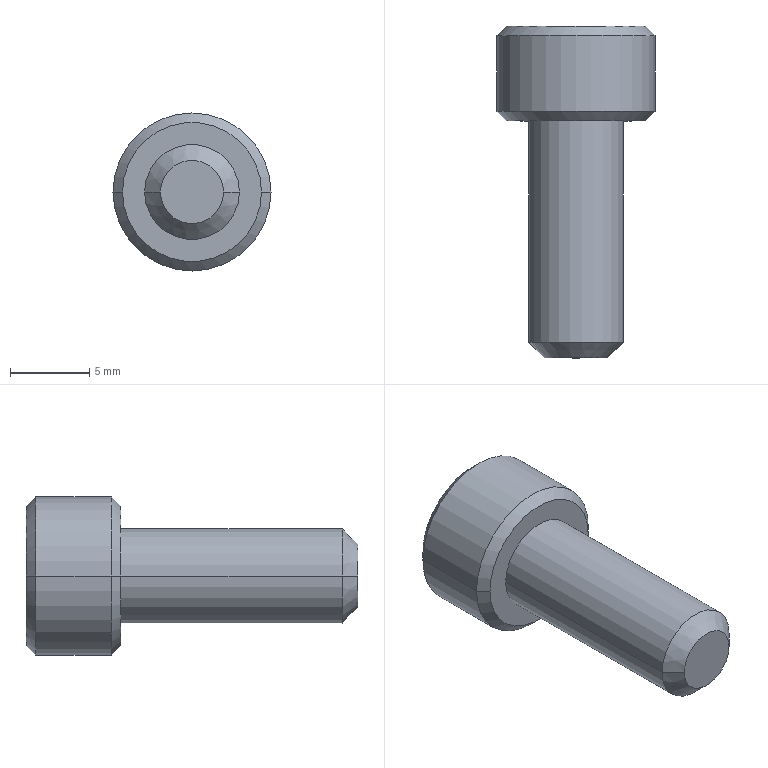Part | STEP file | BB62-M6-15L-7 | 1 solid | 27 faces | box 10 x 21 x 10 mm | volume 798.222 mm3 | plane 15 | cone 8 | cylinder 4 | commonest cylinder face diameters 6 x2 10 x2
STEP:
#1=CARTESIAN_POINT('',(0.,1.349,0.));
#2=VERTEX_POINT('',#1);
#3=CARTESIAN_POINT('',(2.86,3.,0.));
#4=VERTEX_POINT('',#3);
#5=CARTESIAN_POINT('',(0.,1.349,0.));
#6=DIRECTION('',(0.866,0.5,0.));
#7=VECTOR('',#6,1000.);
#8=LINE('',#5,#7);
#9=EDGE_CURVE('',#2,#4,#8,.T.);
#10=ORIENTED_EDGE('',*,*,#9,.F.);
#11=CARTESIAN_POINT('',(-2.86,3.,0.));
#12=VERTEX_POINT('',#11);
#13=CARTESIAN_POINT('',(0.,1.349,0.));
#14=DIRECTION('',(-0.866,0.5,0.));
#15=VECTOR('',#14,1000.);
#16=LINE('',#13,#15);
#17=EDGE_CURVE('',#2,#12,#16,.T.);
#18=ORIENTED_EDGE('',*,*,#17,.T.);
#19=CARTESIAN_POINT('',(-2.477,3.,1.43));
#20=VERTEX_POINT('',#19);
#21=CARTESIAN_POINT('',(0.,3.,0.));
#22=DIRECTION('',(0.,-1.,0.));
#23=DIRECTION('',(-1.,0.,0.));
#24=AXIS2_PLACEMENT_3D('',#21,#22,#23);
#25=CIRCLE('',#24,2.86);
#26=EDGE_CURVE('',#20,#12,#25,.T.);
#27=ORIENTED_EDGE('',*,*,#26,.F.);
#28=CARTESIAN_POINT('',(0.,3.,2.86));
#29=VERTEX_POINT('',#28);
#30=CARTESIAN_POINT('',(0.,3.,0.));
#31=DIRECTION('',(0.,-1.,0.));
#32=DIRECTION('',(-1.,0.,0.));
#33=AXIS2_PLACEMENT_3D('',#30,#31,#32);
#34=CIRCLE('',#33,2.86);
#35=EDGE_CURVE('',#29,#20,#34,.T.);
#36=ORIENTED_EDGE('',*,*,#35,.F.);
#37=CARTESIAN_POINT('',(2.477,3.,1.43));
#38=VERTEX_POINT('',#37);
#39=CARTESIAN_POINT('',(0.,3.,0.));
#40=DIRECTION('',(0.,-1.,0.));
#41=DIRECTION('',(-1.,0.,0.));
#42=AXIS2_PLACEMENT_3D('',#39,#40,#41);
#43=CIRCLE('',#42,2.86);
#44=EDGE_CURVE('',#38,#29,#43,.T.);
#45=ORIENTED_EDGE('',*,*,#44,.F.);
#46=CARTESIAN_POINT('',(0.,3.,0.));
#47=DIRECTION('',(0.,-1.,0.));
#48=DIRECTION('',(-1.,0.,0.));
#49=AXIS2_PLACEMENT_3D('',#46,#47,#48);
#50=CIRCLE('',#49,2.86);
#51=EDGE_CURVE('',#4,#38,#50,.T.);
#52=ORIENTED_EDGE('',*,*,#51,.F.);
#53=EDGE_LOOP('',(#10,#18,#27,#36,#45,#52));
#54=FACE_OUTER_BOUND('',#53,.T.);
#55=CARTESIAN_POINT('',(0.,1001.349,0.));
#56=DIRECTION('',(0.,1.,0.));
#57=DIRECTION('',(1.,0.,0.));
#58=AXIS2_PLACEMENT_3D('',#55,#56,#57);
#59=CONICAL_SURFACE('',#58,1732.051,1.047);
#60=ADVANCED_FACE('',(#54),#59,.F.);
#61=CARTESIAN_POINT('',(2.,-15.,0.));
#62=VERTEX_POINT('',#61);
#63=CARTESIAN_POINT('',(-2.,-15.,0.));
#64=VERTEX_POINT('',#63);
#65=CARTESIAN_POINT('',(0.,-15.,0.));
#66=DIRECTION('',(0.,1.,0.));
#67=DIRECTION('',(1.,0.,0.));
#68=AXIS2_PLACEMENT_3D('',#65,#66,#67);
#69=CIRCLE('',#68,2.);
#70=EDGE_CURVE('',#62,#64,#69,.T.);
#71=ORIENTED_EDGE('',*,*,#70,.T.);
#72=CARTESIAN_POINT('',(-3.,-14.,0.));
#73=VERTEX_POINT('',#72);
#74=CARTESIAN_POINT('',(-2.,-15.,0.));
#75=DIRECTION('',(-0.7071,0.7071,0.));
#76=VECTOR('',#75,1000.);
#77=LINE('',#74,#76);
#78=EDGE_CURVE('',#64,#73,#77,.T.);
#79=ORIENTED_EDGE('',*,*,#78,.T.);
#80=CARTESIAN_POINT('',(3.,-14.,0.));
#81=VERTEX_POINT('',#80);
#82=CARTESIAN_POINT('',(0.,-14.,0.));
#83=DIRECTION('',(0.,-1.,0.));
#84=DIRECTION('',(-1.,0.,0.));
#85=AXIS2_PLACEMENT_3D('',#82,#83,#84);
#86=CIRCLE('',#85,3.);
#87=EDGE_CURVE('',#73,#81,#86,.T.);
#88=ORIENTED_EDGE('',*,*,#87,.T.);
#89=CARTESIAN_POINT('',(2.,-15.,0.));
#90=DIRECTION('',(0.7071,0.7071,0.));
#91=VECTOR('',#90,1000.);
#92=LINE('',#89,#91);
#93=EDGE_CURVE('',#62,#81,#92,.T.);
#94=ORIENTED_EDGE('',*,*,#93,.F.);
#95=EDGE_LOOP('',(#71,#79,#88,#94));
#96=FACE_OUTER_BOUND('',#95,.T.);
#97=CARTESIAN_POINT('',(0.,-15.,0.));
#98=DIRECTION('',(0.,1.,0.));
#99=DIRECTION('',(1.,0.,0.));
#100=AXIS2_PLACEMENT_3D('',#97,#98,#99);
#101=CONICAL_SURFACE('',#100,2.,0.7854);
#102=ADVANCED_FACE('',(#96),#101,.T.);
#103=ORIENTED_EDGE('',*,*,#87,.F.);
#104=CARTESIAN_POINT('',(-3.,0.,0.));
#105=VERTEX_POINT('',#104);
#106=CARTESIAN_POINT('',(-3.,-14.,0.));
#107=DIRECTION('',(0.,1.,0.));
#108=VECTOR('',#107,1000.);
#109=LINE('',#106,#108);
#110=EDGE_CURVE('',#73,#105,#109,.T.);
#111=ORIENTED_EDGE('',*,*,#110,.T.);
#112=CARTESIAN_POINT('',(3.,0.,0.));
#113=VERTEX_POINT('',#112);
#114=CARTESIAN_POINT('',(0.,0.,0.));
#115=DIRECTION('',(0.,-1.,0.));
#116=DIRECTION('',(-1.,0.,0.));
#117=AXIS2_PLACEMENT_3D('',#114,#115,#116);
#118=CIRCLE('',#117,3.);
#119=EDGE_CURVE('',#105,#113,#118,.T.);
#120=ORIENTED_EDGE('',*,*,#119,.T.);
#121=CARTESIAN_POINT('',(3.,-14.,0.));
#122=DIRECTION('',(0.,1.,0.));
#123=VECTOR('',#122,1000.);
#124=LINE('',#121,#123);
#125=EDGE_CURVE('',#81,#113,#124,.T.);
#126=ORIENTED_EDGE('',*,*,#125,.F.);
#127=EDGE_LOOP('',(#103,#111,#120,#126));
#128=FACE_OUTER_BOUND('',#127,.T.);
#129=CARTESIAN_POINT('',(0.,-14.,0.));
#130=DIRECTION('',(0.,1.,0.));
#131=DIRECTION('',(1.,0.,0.));
#132=AXIS2_PLACEMENT_3D('',#129,#130,#131);
#133=CYLINDRICAL_SURFACE('',#132,3.);
#134=ADVANCED_FACE('',(#128),#133,.T.);
#135=CARTESIAN_POINT('',(-4.4,6.,0.));
#136=VERTEX_POINT('',#135);
#137=CARTESIAN_POINT('',(4.4,6.,0.));
#138=VERTEX_POINT('',#137);
#139=CARTESIAN_POINT('',(0.,6.,0.));
#140=DIRECTION('',(0.,-1.,0.));
#141=DIRECTION('',(-1.,0.,0.));
#142=AXIS2_PLACEMENT_3D('',#139,#140,#141);
#143=CIRCLE('',#142,4.4);
#144=EDGE_CURVE('',#136,#138,#143,.T.);
#145=ORIENTED_EDGE('',*,*,#144,.T.);
#146=CARTESIAN_POINT('',(5.,5.4,0.));
#147=VERTEX_POINT('',#146);
#148=CARTESIAN_POINT('',(5.,5.4,0.));
#149=DIRECTION('',(0.7071,-0.7071,0.));
#150=VECTOR('',#149,1000.);
#151=LINE('',#148,#150);
#152=EDGE_CURVE('',#138,#147,#151,.T.);
#153=ORIENTED_EDGE('',*,*,#152,.T.);
#154=CARTESIAN_POINT('',(-5.,5.4,0.));
#155=VERTEX_POINT('',#154);
#156=CARTESIAN_POINT('',(0.,5.4,0.));
#157=DIRECTION('',(0.,-1.,0.));
#158=DIRECTION('',(-1.,0.,0.));
#159=AXIS2_PLACEMENT_3D('',#156,#157,#158);
#160=CIRCLE('',#159,5.);
#161=EDGE_CURVE('',#155,#147,#160,.T.);
#162=ORIENTED_EDGE('',*,*,#161,.F.);
#163=CARTESIAN_POINT('',(-5.,5.4,0.));
#164=DIRECTION('',(-0.7071,-0.7071,0.));
#165=VECTOR('',#164,1000.);
#166=LINE('',#163,#165);
#167=EDGE_CURVE('',#136,#155,#166,.T.);
#168=ORIENTED_EDGE('',*,*,#167,.F.);
#169=EDGE_LOOP('',(#145,#153,#162,#168));
#170=FACE_OUTER_BOUND('',#169,.T.);
#171=CARTESIAN_POINT('',(0.,5.4,0.));
#172=DIRECTION('',(0.,-1.,0.));
#173=DIRECTION('',(-1.,0.,0.));
#174=AXIS2_PLACEMENT_3D('',#171,#172,#173);
#175=CONICAL_SURFACE('',#174,5.,0.7854);
#176=ADVANCED_FACE('',(#170),#175,.T.);
#177=ORIENTED_EDGE('',*,*,#161,.T.);
#178=CARTESIAN_POINT('',(5.,0.6,0.));
#179=VERTEX_POINT('',#178);
#180=CARTESIAN_POINT('',(5.,1.62,0.));
#181=DIRECTION('',(0.,-1.,0.));
#182=VECTOR('',#181,1000.);
#183=LINE('',#180,#182);
#184=EDGE_CURVE('',#147,#179,#183,.T.);
#185=ORIENTED_EDGE('',*,*,#184,.T.);
#186=CARTESIAN_POINT('',(-5.,0.6,0.));
#187=VERTEX_POINT('',#186);
#188=CARTESIAN_POINT('',(0.,0.6,0.));
#189=DIRECTION('',(0.,-1.,0.));
#190=DIRECTION('',(-1.,0.,0.));
#191=AXIS2_PLACEMENT_3D('',#188,#189,#190);
#192=CIRCLE('',#191,5.);
#193=EDGE_CURVE('',#187,#179,#192,.T.);
#194=ORIENTED_EDGE('',*,*,#193,.F.);
#195=CARTESIAN_POINT('',(-5.,1.62,0.));
#196=DIRECTION('',(0.,-1.,0.));
#197=VECTOR('',#196,1000.);
#198=LINE('',#195,#197);
#199=EDGE_CURVE('',#155,#187,#198,.T.);
#200=ORIENTED_EDGE('',*,*,#199,.F.);
#201=EDGE_LOOP('',(#177,#185,#194,#200));
#202=FACE_OUTER_BOUND('',#201,.T.);
#203=CARTESIAN_POINT('',(0.,1.62,0.));
#204=DIRECTION('',(0.,-1.,0.));
#205=DIRECTION('',(-1.,0.,0.));
#206=AXIS2_PLACEMENT_3D('',#203,#204,#205);
#207=CYLINDRICAL_SURFACE('',#206,5.);
#208=ADVANCED_FACE('',(#202),#207,.T.);
#209=CARTESIAN_POINT('',(-4.4,0.,0.));
#210=VERTEX_POINT('',#209);
#211=CARTESIAN_POINT('',(4.4,0.,0.));
#212=VERTEX_POINT('',#211);
#213=CARTESIAN_POINT('',(0.,0.,0.));
#214=DIRECTION('',(0.,-1.,0.));
#215=DIRECTION('',(-1.,0.,0.));
#216=AXIS2_PLACEMENT_3D('',#213,#214,#215);
#217=CIRCLE('',#216,4.4);
#218=EDGE_CURVE('',#210,#212,#217,.T.);
#219=ORIENTED_EDGE('',*,*,#218,.F.);
#220=CARTESIAN_POINT('',(-4.4,0.,0.));
#221=DIRECTION('',(-0.7071,0.7071,0.));
#222=VECTOR('',#221,1000.);
#223=LINE('',#220,#222);
#224=EDGE_CURVE('',#210,#187,#223,.T.);
#225=ORIENTED_EDGE('',*,*,#224,.T.);
#226=ORIENTED_EDGE('',*,*,#193,.T.);
#227=CARTESIAN_POINT('',(4.4,0.,0.));
#228=DIRECTION('',(0.7071,0.7071,0.));
#229=VECTOR('',#228,1000.);
#230=LINE('',#227,#229);
#231=EDGE_CURVE('',#212,#179,#230,.T.);
#232=ORIENTED_EDGE('',*,*,#231,.F.);
#233=EDGE_LOOP('',(#219,#225,#226,#232));
#234=FACE_OUTER_BOUND('',#233,.T.);
#235=CARTESIAN_POINT('',(0.,0.,0.));
#236=DIRECTION('',(0.,1.,0.));
#237=DIRECTION('',(1.,0.,0.));
#238=AXIS2_PLACEMENT_3D('',#235,#236,#237);
#239=CONICAL_SURFACE('',#238,4.4,0.7854);
#240=ADVANCED_FACE('',(#234),#239,.T.);
#241=ORIENTED_EDGE('',*,*,#144,.F.);
#242=CARTESIAN_POINT('',(0.,6.,0.));
#243=DIRECTION('',(0.,-1.,0.));
#244=DIRECTION('',(-1.,0.,0.));
#245=AXIS2_PLACEMENT_3D('',#242,#243,#244);
#246=CIRCLE('',#245,4.4);
#247=EDGE_CURVE('',#138,#136,#246,.T.);
#248=ORIENTED_EDGE('',*,*,#247,.F.);
#249=EDGE_LOOP('',(#241,#248));
#250=FACE_OUTER_BOUND('',#249,.T.);
#251=CARTESIAN_POINT('',(0.,6.,-2.86));
#252=VERTEX_POINT('',#251);
#253=CARTESIAN_POINT('',(-2.477,6.,-1.43));
#254=VERTEX_POINT('',#253);
#255=CARTESIAN_POINT('',(0.,6.,-2.86));
#256=DIRECTION('',(-0.866,0.,0.5));
#257=VECTOR('',#256,1000.);
#258=LINE('',#255,#257);
#259=EDGE_CURVE('',#252,#254,#258,.T.);
#260=ORIENTED_EDGE('',*,*,#259,.F.);
#261=CARTESIAN_POINT('',(2.477,6.,-1.43));
#262=VERTEX_POINT('',#261);
#263=CARTESIAN_POINT('',(2.477,6.,-1.43));
#264=DIRECTION('',(-0.866,0.,-0.5));
#265=VECTOR('',#264,1000.);
#266=LINE('',#263,#265);
#267=EDGE_CURVE('',#262,#252,#266,.T.);
#268=ORIENTED_EDGE('',*,*,#267,.F.);
#269=CARTESIAN_POINT('',(2.477,6.,1.43));
#270=VERTEX_POINT('',#269);
#271=CARTESIAN_POINT('',(2.477,6.,1.43));
#272=DIRECTION('',(0.,0.,-1.));
#273=VECTOR('',#272,1000.);
#274=LINE('',#271,#273);
#275=EDGE_CURVE('',#270,#262,#274,.T.);
#276=ORIENTED_EDGE('',*,*,#275,.F.);
#277=CARTESIAN_POINT('',(0.,6.,2.86));
#278=VERTEX_POINT('',#277);
#279=CARTESIAN_POINT('',(0.,6.,2.86));
#280=DIRECTION('',(0.866,0.,-0.5));
#281=VECTOR('',#280,1000.);
#282=LINE('',#279,#281);
#283=EDGE_CURVE('',#278,#270,#282,.T.);
#284=ORIENTED_EDGE('',*,*,#283,.F.);
#285=CARTESIAN_POINT('',(-2.477,6.,1.43));
#286=VERTEX_POINT('',#285);
#287=CARTESIAN_POINT('',(-2.477,6.,1.43));
#288=DIRECTION('',(0.866,0.,0.5));
#289=VECTOR('',#288,1000.);
#290=LINE('',#287,#289);
#291=EDGE_CURVE('',#286,#278,#290,.T.);
#292=ORIENTED_EDGE('',*,*,#291,.F.);
#293=CARTESIAN_POINT('',(-2.477,6.,-1.43));
#294=DIRECTION('',(0.,0.,1.));
#295=VECTOR('',#294,1000.);
#296=LINE('',#293,#295);
#297=EDGE_CURVE('',#254,#286,#296,.T.);
#298=ORIENTED_EDGE('',*,*,#297,.F.);
#299=EDGE_LOOP('',(#260,#268,#276,#284,#292,#298));
#300=FACE_BOUND('',#299,.T.);
#301=CARTESIAN_POINT('',(4.4,6.,0.));
#302=DIRECTION('',(0.,1.,0.));
#303=DIRECTION('',(1.,0.,0.));
#304=AXIS2_PLACEMENT_3D('',#301,#302,#303);
#305=PLANE('',#304);
#306=ADVANCED_FACE('',(#250,#300),#305,.T.);
#307=CARTESIAN_POINT('',(0.,0.,0.));
#308=DIRECTION('',(0.,-1.,0.));
#309=DIRECTION('',(-1.,0.,0.));
#310=AXIS2_PLACEMENT_3D('',#307,#308,#309);
#311=CIRCLE('',#310,3.);
#312=EDGE_CURVE('',#113,#105,#311,.T.);
#313=ORIENTED_EDGE('',*,*,#312,.F.);
#314=ORIENTED_EDGE('',*,*,#119,.F.);
#315=EDGE_LOOP('',(#313,#314));
#316=FACE_BOUND('',#315,.T.);
#317=CARTESIAN_POINT('',(0.,0.,0.));
#318=DIRECTION('',(0.,-1.,0.));
#319=DIRECTION('',(-1.,0.,0.));
#320=AXIS2_PLACEMENT_3D('',#317,#318,#319);
#321=CIRCLE('',#320,4.4);
#322=EDGE_CURVE('',#212,#210,#321,.T.);
#323=ORIENTED_EDGE('',*,*,#322,.T.);
#324=ORIENTED_EDGE('',*,*,#218,.T.);
#325=EDGE_LOOP('',(#323,#324));
#326=FACE_OUTER_BOUND('',#325,.T.);
#327=CARTESIAN_POINT('',(0.,0.,0.));
#328=DIRECTION('',(0.,-1.,0.));
#329=DIRECTION('',(-1.,0.,0.));
#330=AXIS2_PLACEMENT_3D('',#327,#328,#329);
#331=PLANE('',#330);
#332=ADVANCED_FACE('',(#316,#326),#331,.T.);
#333=ORIENTED_EDGE('',*,*,#224,.F.);
#334=ORIENTED_EDGE('',*,*,#322,.F.);
#335=ORIENTED_EDGE('',*,*,#231,.T.);
#336=CARTESIAN_POINT('',(0.,0.6,0.));
#337=DIRECTION('',(0.,-1.,0.));
#338=DIRECTION('',(-1.,0.,0.));
#339=AXIS2_PLACEMENT_3D('',#336,#337,#338);
#340=CIRCLE('',#339,5.);
#341=EDGE_CURVE('',#179,#187,#340,.T.);
#342=ORIENTED_EDGE('',*,*,#341,.T.);
#343=EDGE_LOOP('',(#333,#334,#335,#342));
#344=FACE_OUTER_BOUND('',#343,.T.);
#345=CARTESIAN_POINT('',(0.,0.,0.));
#346=DIRECTION('',(0.,1.,0.));
#347=DIRECTION('',(1.,0.,0.));
#348=AXIS2_PLACEMENT_3D('',#345,#346,#347);
#349=CONICAL_SURFACE('',#348,4.4,0.7854);
#350=ADVANCED_FACE('',(#344),#349,.T.);
#351=ORIENTED_EDGE('',*,*,#184,.F.);
#352=CARTESIAN_POINT('',(0.,5.4,0.));
#353=DIRECTION('',(0.,-1.,0.));
#354=DIRECTION('',(-1.,0.,0.));
#355=AXIS2_PLACEMENT_3D('',#352,#353,#354);
#356=CIRCLE('',#355,5.);
#357=EDGE_CURVE('',#147,#155,#356,.T.);
#358=ORIENTED_EDGE('',*,*,#357,.T.);
#359=ORIENTED_EDGE('',*,*,#199,.T.);
#360=ORIENTED_EDGE('',*,*,#341,.F.);
#361=EDGE_LOOP('',(#351,#358,#359,#360));
#362=FACE_OUTER_BOUND('',#361,.T.);
#363=CARTESIAN_POINT('',(0.,1.62,0.));
#364=DIRECTION('',(0.,-1.,0.));
#365=DIRECTION('',(-1.,0.,0.));
#366=AXIS2_PLACEMENT_3D('',#363,#364,#365);
#367=CYLINDRICAL_SURFACE('',#366,5.);
#368=ADVANCED_FACE('',(#362),#367,.T.);
#369=ORIENTED_EDGE('',*,*,#152,.F.);
#370=ORIENTED_EDGE('',*,*,#247,.T.);
#371=ORIENTED_EDGE('',*,*,#167,.T.);
#372=ORIENTED_EDGE('',*,*,#357,.F.);
#373=EDGE_LOOP('',(#369,#370,#371,#372));
#374=FACE_OUTER_BOUND('',#373,.T.);
#375=CARTESIAN_POINT('',(0.,5.4,0.));
#376=DIRECTION('',(0.,-1.,0.));
#377=DIRECTION('',(-1.,0.,0.));
#378=AXIS2_PLACEMENT_3D('',#375,#376,#377);
#379=CONICAL_SURFACE('',#378,5.,0.7854);
#380=ADVANCED_FACE('',(#374),#379,.T.);
#381=ORIENTED_EDGE('',*,*,#110,.F.);
#382=CARTESIAN_POINT('',(0.,-14.,0.));
#383=DIRECTION('',(0.,-1.,0.));
#384=DIRECTION('',(-1.,0.,0.));
#385=AXIS2_PLACEMENT_3D('',#382,#383,#384);
#386=CIRCLE('',#385,3.);
#387=EDGE_CURVE('',#81,#73,#386,.T.);
#388=ORIENTED_EDGE('',*,*,#387,.F.);
#389=ORIENTED_EDGE('',*,*,#125,.T.);
#390=ORIENTED_EDGE('',*,*,#312,.T.);
#391=EDGE_LOOP('',(#381,#388,#389,#390));
#392=FACE_OUTER_BOUND('',#391,.T.);
#393=CARTESIAN_POINT('',(0.,-14.,0.));
#394=DIRECTION('',(0.,1.,0.));
#395=DIRECTION('',(1.,0.,0.));
#396=AXIS2_PLACEMENT_3D('',#393,#394,#395);
#397=CYLINDRICAL_SURFACE('',#396,3.);
#398=ADVANCED_FACE('',(#392),#397,.T.);
#399=ORIENTED_EDGE('',*,*,#70,.F.);
#400=CARTESIAN_POINT('',(0.,-15.,0.));
#401=DIRECTION('',(0.,1.,0.));
#402=DIRECTION('',(1.,0.,0.));
#403=AXIS2_PLACEMENT_3D('',#400,#401,#402);
#404=CIRCLE('',#403,2.);
#405=EDGE_CURVE('',#64,#62,#404,.T.);
#406=ORIENTED_EDGE('',*,*,#405,.F.);
#407=EDGE_LOOP('',(#399,#406));
#408=FACE_OUTER_BOUND('',#407,.T.);
#409=CARTESIAN_POINT('',(0.,-15.,0.));
#410=DIRECTION('',(0.,-1.,0.));
#411=DIRECTION('',(-1.,0.,0.));
#412=AXIS2_PLACEMENT_3D('',#409,#410,#411);
#413=PLANE('',#412);
#414=ADVANCED_FACE('',(#408),#413,.T.);
#415=ORIENTED_EDGE('',*,*,#78,.F.);
#416=ORIENTED_EDGE('',*,*,#405,.T.);
#417=ORIENTED_EDGE('',*,*,#93,.T.);
#418=ORIENTED_EDGE('',*,*,#387,.T.);
#419=EDGE_LOOP('',(#415,#416,#417,#418));
#420=FACE_OUTER_BOUND('',#419,.T.);
#421=CARTESIAN_POINT('',(0.,-15.,0.));
#422=DIRECTION('',(0.,1.,0.));
#423=DIRECTION('',(1.,0.,0.));
#424=AXIS2_PLACEMENT_3D('',#421,#422,#423);
#425=CONICAL_SURFACE('',#424,2.,0.7854);
#426=ADVANCED_FACE('',(#420),#425,.T.);
#427=CARTESIAN_POINT('',(2.477,3.,-1.43));
#428=VERTEX_POINT('',#427);
#429=CARTESIAN_POINT('',(0.,3.,-2.86));
#430=VERTEX_POINT('',#429);
#431=CARTESIAN_POINT('',(2.477,3.,-1.43));
#432=DIRECTION('',(-0.866,0.,-0.5));
#433=VECTOR('',#432,1000.);
#434=LINE('',#431,#433);
#435=EDGE_CURVE('',#428,#430,#434,.T.);
#436=ORIENTED_EDGE('',*,*,#435,.F.);
#437=CARTESIAN_POINT('',(2.477,6.,-1.43));
#438=DIRECTION('',(0.,-1.,0.));
#439=VECTOR('',#438,1000.);
#440=LINE('',#437,#439);
#441=EDGE_CURVE('',#262,#428,#440,.T.);
#442=ORIENTED_EDGE('',*,*,#441,.F.);
#443=ORIENTED_EDGE('',*,*,#267,.T.);
#444=CARTESIAN_POINT('',(0.,6.,-2.86));
#445=DIRECTION('',(0.,-1.,0.));
#446=VECTOR('',#445,1000.);
#447=LINE('',#444,#446);
#448=EDGE_CURVE('',#252,#430,#447,.T.);
#449=ORIENTED_EDGE('',*,*,#448,.T.);
#450=EDGE_LOOP('',(#436,#442,#443,#449));
#451=FACE_OUTER_BOUND('',#450,.T.);
#452=CARTESIAN_POINT('',(2.477,6.,-1.43));
#453=DIRECTION('',(-0.5,0.,0.866));
#454=DIRECTION('',(0.866,0.,0.5));
#455=AXIS2_PLACEMENT_3D('',#452,#453,#454);
#456=PLANE('',#455);
#457=ADVANCED_FACE('',(#451),#456,.T.);
#458=CARTESIAN_POINT('',(-2.477,3.,-1.43));
#459=VERTEX_POINT('',#458);
#460=CARTESIAN_POINT('',(0.,3.,-2.86));
#461=DIRECTION('',(-0.866,0.,0.5));
#462=VECTOR('',#461,1000.);
#463=LINE('',#460,#462);
#464=EDGE_CURVE('',#430,#459,#463,.T.);
#465=ORIENTED_EDGE('',*,*,#464,.F.);
#466=ORIENTED_EDGE('',*,*,#448,.F.);
#467=ORIENTED_EDGE('',*,*,#259,.T.);
#468=CARTESIAN_POINT('',(-2.477,6.,-1.43));
#469=DIRECTION('',(0.,-1.,0.));
#470=VECTOR('',#469,1000.);
#471=LINE('',#468,#470);
#472=EDGE_CURVE('',#254,#459,#471,.T.);
#473=ORIENTED_EDGE('',*,*,#472,.T.);
#474=EDGE_LOOP('',(#465,#466,#467,#473));
#475=FACE_OUTER_BOUND('',#474,.T.);
#476=CARTESIAN_POINT('',(0.,6.,-2.86));
#477=DIRECTION('',(0.5,0.,0.866));
#478=DIRECTION('',(0.866,0.,-0.5));
#479=AXIS2_PLACEMENT_3D('',#476,#477,#478);
#480=PLANE('',#479);
#481=ADVANCED_FACE('',(#475),#480,.T.);
#482=CARTESIAN_POINT('',(-2.477,3.,-1.43));
#483=DIRECTION('',(0.,0.,1.));
#484=VECTOR('',#483,1000.);
#485=LINE('',#482,#484);
#486=EDGE_CURVE('',#459,#20,#485,.T.);
#487=ORIENTED_EDGE('',*,*,#486,.F.);
#488=ORIENTED_EDGE('',*,*,#472,.F.);
#489=ORIENTED_EDGE('',*,*,#297,.T.);
#490=CARTESIAN_POINT('',(-2.477,6.,1.43));
#491=DIRECTION('',(0.,-1.,0.));
#492=VECTOR('',#491,1000.);
#493=LINE('',#490,#492);
#494=EDGE_CURVE('',#286,#20,#493,.T.);
#495=ORIENTED_EDGE('',*,*,#494,.T.);
#496=EDGE_LOOP('',(#487,#488,#489,#495));
#497=FACE_OUTER_BOUND('',#496,.T.);
#498=CARTESIAN_POINT('',(-2.477,6.,-1.43));
#499=DIRECTION('',(1.,0.,0.));
#500=DIRECTION('',(0.,0.,-1.));
#501=AXIS2_PLACEMENT_3D('',#498,#499,#500);
#502=PLANE('',#501);
#503=ADVANCED_FACE('',(#497),#502,.T.);
#504=CARTESIAN_POINT('',(-2.477,3.,1.43));
#505=DIRECTION('',(0.866,0.,0.5));
#506=VECTOR('',#505,1000.);
#507=LINE('',#504,#506);
#508=EDGE_CURVE('',#20,#29,#507,.T.);
#509=ORIENTED_EDGE('',*,*,#508,.F.);
#510=ORIENTED_EDGE('',*,*,#494,.F.);
#511=ORIENTED_EDGE('',*,*,#291,.T.);
#512=CARTESIAN_POINT('',(0.,6.,2.86));
#513=DIRECTION('',(0.,-1.,0.));
#514=VECTOR('',#513,1000.);
#515=LINE('',#512,#514);
#516=EDGE_CURVE('',#278,#29,#515,.T.);
#517=ORIENTED_EDGE('',*,*,#516,.T.);
#518=EDGE_LOOP('',(#509,#510,#511,#517));
#519=FACE_OUTER_BOUND('',#518,.T.);
#520=CARTESIAN_POINT('',(-2.477,6.,1.43));
#521=DIRECTION('',(0.5,0.,-0.866));
#522=DIRECTION('',(-0.866,0.,-0.5));
#523=AXIS2_PLACEMENT_3D('',#520,#521,#522);
#524=PLANE('',#523);
#525=ADVANCED_FACE('',(#519),#524,.T.);
#526=CARTESIAN_POINT('',(0.,3.,2.86));
#527=DIRECTION('',(0.866,0.,-0.5));
#528=VECTOR('',#527,1000.);
#529=LINE('',#526,#528);
#530=EDGE_CURVE('',#29,#38,#529,.T.);
#531=ORIENTED_EDGE('',*,*,#530,.F.);
#532=ORIENTED_EDGE('',*,*,#516,.F.);
#533=ORIENTED_EDGE('',*,*,#283,.T.);
#534=CARTESIAN_POINT('',(2.477,6.,1.43));
#535=DIRECTION('',(0.,-1.,0.));
#536=VECTOR('',#535,1000.);
#537=LINE('',#534,#536);
#538=EDGE_CURVE('',#270,#38,#537,.T.);
#539=ORIENTED_EDGE('',*,*,#538,.T.);
#540=EDGE_LOOP('',(#531,#532,#533,#539));
#541=FACE_OUTER_BOUND('',#540,.T.);
#542=CARTESIAN_POINT('',(0.,6.,2.86));
#543=DIRECTION('',(-0.5,0.,-0.866));
#544=DIRECTION('',(-0.866,0.,0.5));
#545=AXIS2_PLACEMENT_3D('',#542,#543,#544);
#546=PLANE('',#545);
#547=ADVANCED_FACE('',(#541),#546,.T.);
#548=CARTESIAN_POINT('',(2.477,3.,1.43));
#549=DIRECTION('',(0.,0.,-1.));
#550=VECTOR('',#549,1000.);
#551=LINE('',#548,#550);
#552=EDGE_CURVE('',#38,#428,#551,.T.);
#553=ORIENTED_EDGE('',*,*,#552,.F.);
#554=ORIENTED_EDGE('',*,*,#538,.F.);
#555=ORIENTED_EDGE('',*,*,#275,.T.);
#556=ORIENTED_EDGE('',*,*,#441,.T.);
#557=EDGE_LOOP('',(#553,#554,#555,#556));
#558=FACE_OUTER_BOUND('',#557,.T.);
#559=CARTESIAN_POINT('',(2.477,6.,1.43));
#560=DIRECTION('',(-1.,0.,0.));
#561=DIRECTION('',(0.,0.,1.));
#562=AXIS2_PLACEMENT_3D('',#559,#560,#561);
#563=PLANE('',#562);
#564=ADVANCED_FACE('',(#558),#563,.T.);
#565=ORIENTED_EDGE('',*,*,#435,.T.);
#566=CARTESIAN_POINT('',(0.,3.,0.));
#567=DIRECTION('',(0.,-1.,0.));
#568=DIRECTION('',(-1.,0.,0.));
#569=AXIS2_PLACEMENT_3D('',#566,#567,#568);
#570=CIRCLE('',#569,2.86);
#571=EDGE_CURVE('',#430,#428,#570,.T.);
#572=ORIENTED_EDGE('',*,*,#571,.T.);
#573=EDGE_LOOP('',(#565,#572));
#574=FACE_OUTER_BOUND('',#573,.T.);
#575=CARTESIAN_POINT('',(0.,3.,0.));
#576=DIRECTION('',(0.,1.,0.));
#577=DIRECTION('',(1.,0.,0.));
#578=AXIS2_PLACEMENT_3D('',#575,#576,#577);
#579=PLANE('',#578);
#580=ADVANCED_FACE('',(#574),#579,.F.);
#581=ORIENTED_EDGE('',*,*,#552,.T.);
#582=CARTESIAN_POINT('',(0.,3.,0.));
#583=DIRECTION('',(0.,-1.,0.));
#584=DIRECTION('',(-1.,0.,0.));
#585=AXIS2_PLACEMENT_3D('',#582,#583,#584);
#586=CIRCLE('',#585,2.86);
#587=EDGE_CURVE('',#428,#4,#586,.T.);
#588=ORIENTED_EDGE('',*,*,#587,.T.);
#589=ORIENTED_EDGE('',*,*,#51,.T.);
#590=EDGE_LOOP('',(#581,#588,#589));
#591=FACE_OUTER_BOUND('',#590,.T.);
#592=CARTESIAN_POINT('',(0.,3.,0.));
#593=DIRECTION('',(0.,1.,0.));
#594=DIRECTION('',(1.,0.,0.));
#595=AXIS2_PLACEMENT_3D('',#592,#593,#594);
#596=PLANE('',#595);
#597=ADVANCED_FACE('',(#591),#596,.F.);
#598=ORIENTED_EDGE('',*,*,#530,.T.);
#599=ORIENTED_EDGE('',*,*,#44,.T.);
#600=EDGE_LOOP('',(#598,#599));
#601=FACE_OUTER_BOUND('',#600,.T.);
#602=CARTESIAN_POINT('',(0.,3.,0.));
#603=DIRECTION('',(0.,1.,0.));
#604=DIRECTION('',(1.,0.,0.));
#605=AXIS2_PLACEMENT_3D('',#602,#603,#604);
#606=PLANE('',#605);
#607=ADVANCED_FACE('',(#601),#606,.F.);
#608=ORIENTED_EDGE('',*,*,#508,.T.);
#609=ORIENTED_EDGE('',*,*,#35,.T.);
#610=EDGE_LOOP('',(#608,#609));
#611=FACE_OUTER_BOUND('',#610,.T.);
#612=CARTESIAN_POINT('',(0.,3.,0.));
#613=DIRECTION('',(0.,1.,0.));
#614=DIRECTION('',(1.,0.,0.));
#615=AXIS2_PLACEMENT_3D('',#612,#613,#614);
#616=PLANE('',#615);
#617=ADVANCED_FACE('',(#611),#616,.F.);
#618=ORIENTED_EDGE('',*,*,#486,.T.);
#619=ORIENTED_EDGE('',*,*,#26,.T.);
#620=CARTESIAN_POINT('',(0.,3.,0.));
#621=DIRECTION('',(0.,-1.,0.));
#622=DIRECTION('',(-1.,0.,0.));
#623=AXIS2_PLACEMENT_3D('',#620,#621,#622);
#624=CIRCLE('',#623,2.86);
#625=EDGE_CURVE('',#12,#459,#624,.T.);
#626=ORIENTED_EDGE('',*,*,#625,.T.);
#627=EDGE_LOOP('',(#618,#619,#626));
#628=FACE_OUTER_BOUND('',#627,.T.);
#629=CARTESIAN_POINT('',(0.,3.,0.));
#630=DIRECTION('',(0.,1.,0.));
#631=DIRECTION('',(1.,0.,0.));
#632=AXIS2_PLACEMENT_3D('',#629,#630,#631);
#633=PLANE('',#632);
#634=ADVANCED_FACE('',(#628),#633,.F.);
#635=ORIENTED_EDGE('',*,*,#464,.T.);
#636=CARTESIAN_POINT('',(0.,3.,0.));
#637=DIRECTION('',(0.,-1.,0.));
#638=DIRECTION('',(-1.,0.,0.));
#639=AXIS2_PLACEMENT_3D('',#636,#637,#638);
#640=CIRCLE('',#639,2.86);
#641=EDGE_CURVE('',#459,#430,#640,.T.);
#642=ORIENTED_EDGE('',*,*,#641,.T.);
#643=EDGE_LOOP('',(#635,#642));
#644=FACE_OUTER_BOUND('',#643,.T.);
#645=CARTESIAN_POINT('',(0.,3.,0.));
#646=DIRECTION('',(0.,1.,0.));
#647=DIRECTION('',(1.,0.,0.));
#648=AXIS2_PLACEMENT_3D('',#645,#646,#647);
#649=PLANE('',#648);
#650=ADVANCED_FACE('',(#644),#649,.F.);
#651=ORIENTED_EDGE('',*,*,#17,.F.);
#652=ORIENTED_EDGE('',*,*,#9,.T.);
#653=ORIENTED_EDGE('',*,*,#587,.F.);
#654=ORIENTED_EDGE('',*,*,#571,.F.);
#655=ORIENTED_EDGE('',*,*,#641,.F.);
#656=ORIENTED_EDGE('',*,*,#625,.F.);
#657=EDGE_LOOP('',(#651,#652,#653,#654,#655,#656));
#658=FACE_OUTER_BOUND('',#657,.T.);
#659=CARTESIAN_POINT('',(0.,1001.349,0.));
#660=DIRECTION('',(0.,1.,0.));
#661=DIRECTION('',(1.,0.,0.));
#662=AXIS2_PLACEMENT_3D('',#659,#660,#661);
#663=CONICAL_SURFACE('',#662,1732.051,1.047);
#664=ADVANCED_FACE('',(#658),#663,.F.);
#665=CLOSED_SHELL('',(#60,#102,#134,#176,#208,#240,#306,#332,#350,#368,#380,#398,#414,#426,#457,#481,#503,#525,#547,#564,#580,#597,#607,#617,#634,#650,#664));
#666=MANIFOLD_SOLID_BREP('',#665);
#667=CARTESIAN_POINT('',(0.,0.,0.));
#668=DIRECTION('',(0.,0.,1.));
#669=DIRECTION('',(1.,0.,0.));
#670=AXIS2_PLACEMENT_3D('',#667,#668,#669);
#671=(LENGTH_UNIT()NAMED_UNIT(*)SI_UNIT(.MILLI.,.METRE.));
#672=UNCERTAINTY_MEASURE_WITH_UNIT(LENGTH_MEASURE(0.00001),#671,'','');
#673=(NAMED_UNIT(*)PLANE_ANGLE_UNIT()SI_UNIT($,.RADIAN.));
#674=(NAMED_UNIT(*)SI_UNIT($,.STERADIAN.)SOLID_ANGLE_UNIT());
#675=(GEOMETRIC_REPRESENTATION_CONTEXT(3)GLOBAL_UNCERTAINTY_ASSIGNED_CONTEXT((#672))GLOBAL_UNIT_ASSIGNED_CONTEXT((#671,#673,#674))REPRESENTATION_CONTEXT('',''));
#676=ADVANCED_BREP_SHAPE_REPRESENTATION('',(#666,#670),#675);